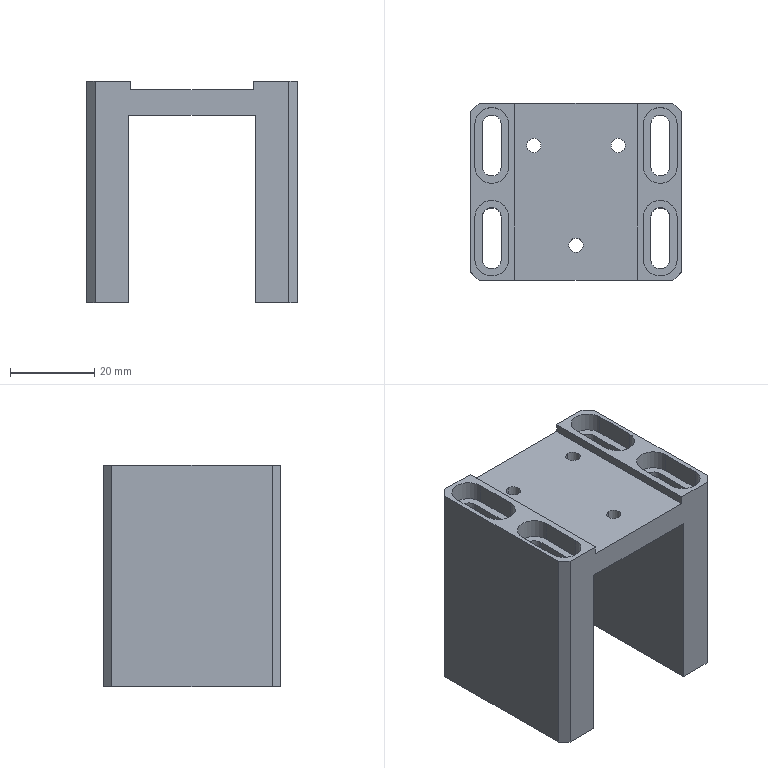Part | SolidWorks | features HoleWzd 2, ICE 2, Chamfer 1, Extrusion 1 | 1 solid | 60 faces | box 50 x 42 x 52.5 mm | volume 37086 mm3 | plane 38 | cylinder 22 | commonest cylinder face diameters 4.5 x8 8 x8 3.4 x6